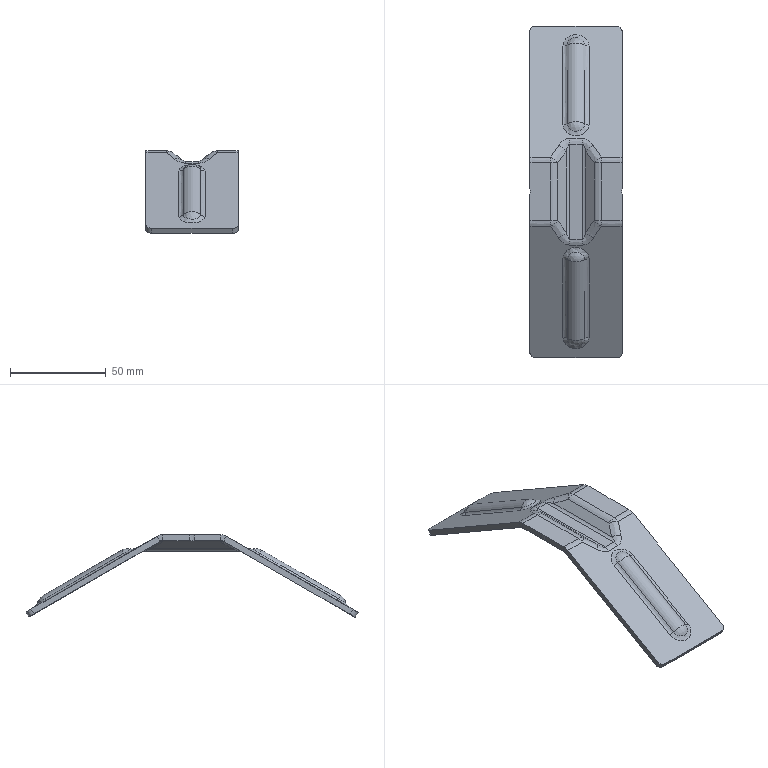Part | STEP file | 1_id86_x_t | 1 solid | 108 faces | box 48 x 173.045 x 42.999 mm | volume 28624 mm3 | spline 58 | plane 20 | sphere 16 | cylinder 14 | commonest cylinder face diameters 5.85 x2 6 x2 6.3 x2 9.576 x2 11.85 x2 12 x2